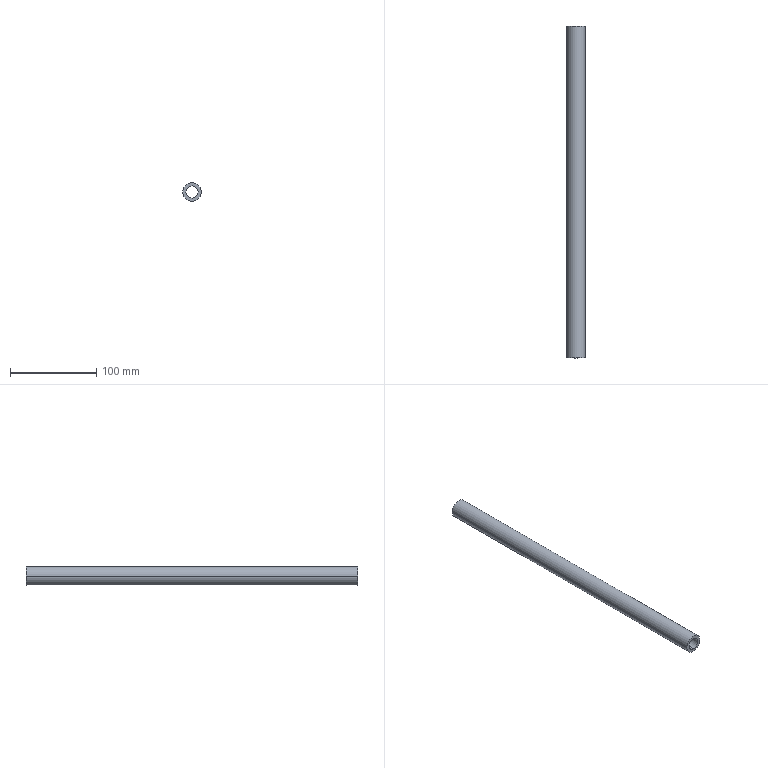Part | SolidWorks | features BaseBody 1 | 1 solid | 6 faces | box 21.234 x 384.346 x 21.234 mm | volume 76950 mm3 | plane 2 | spline 2 | cylinder 2 | commonest cylinder face diameters 21.234 x2
STEP:
#1=CARTESIAN_POINT('',(-35.306,422.7,7.));
#2=VERTEX_POINT('',#1);
#3=CARTESIAN_POINT('',(-35.306,422.7,-7.));
#4=VERTEX_POINT('',#3);
#5=CARTESIAN_POINT('',(-35.306,422.7,7.));
#6=CARTESIAN_POINT('',(-35.791,422.7,7.));
#7=CARTESIAN_POINT('',(-36.275,422.7,6.95));
#8=CARTESIAN_POINT('',(-36.75,422.7,6.85));
#9=CARTESIAN_POINT('',(-37.321,422.7,6.729));
#10=CARTESIAN_POINT('',(-37.875,422.7,6.538));
#11=CARTESIAN_POINT('',(-38.399,422.7,6.28));
#12=CARTESIAN_POINT('',(-39.149,422.7,5.91));
#13=CARTESIAN_POINT('',(-39.828,422.7,5.409));
#14=CARTESIAN_POINT('',(-40.401,422.7,4.8));
#15=CARTESIAN_POINT('',(-40.996,422.7,4.168));
#16=CARTESIAN_POINT('',(-41.469,422.7,3.431));
#17=CARTESIAN_POINT('',(-41.794,422.7,2.626));
#18=CARTESIAN_POINT('',(-42.132,422.7,1.792));
#19=CARTESIAN_POINT('',(-42.306,422.7,0.9002));
#20=CARTESIAN_POINT('',(-42.306,422.7,0.));
#21=CARTESIAN_POINT('',(-42.306,422.7,-0.9002));
#22=CARTESIAN_POINT('',(-42.132,422.7,-1.792));
#23=CARTESIAN_POINT('',(-41.794,422.7,-2.626));
#24=CARTESIAN_POINT('',(-41.469,422.7,-3.431));
#25=CARTESIAN_POINT('',(-40.996,422.7,-4.168));
#26=CARTESIAN_POINT('',(-40.401,422.7,-4.8));
#27=CARTESIAN_POINT('',(-39.828,422.7,-5.409));
#28=CARTESIAN_POINT('',(-39.149,422.7,-5.91));
#29=CARTESIAN_POINT('',(-38.399,422.7,-6.28));
#30=CARTESIAN_POINT('',(-37.875,422.7,-6.538));
#31=CARTESIAN_POINT('',(-37.321,422.7,-6.729));
#32=CARTESIAN_POINT('',(-36.75,422.7,-6.85));
#33=CARTESIAN_POINT('',(-36.275,422.7,-6.95));
#34=CARTESIAN_POINT('',(-35.791,422.7,-7.));
#35=CARTESIAN_POINT('',(-35.306,422.7,-7.));
#36=B_SPLINE_CURVE_WITH_KNOTS('',3,(#5,#6,#7,#8,#9,#10,#11,#12,#13,#14,#15,#16,#17,#18,#19,#20,#21,#22,#23,#24,#25,#26,#27,#28,#29,#30,#31,#32,#33,#34,#35),.UNSPECIFIED.,.F.,.F.,(4,3,3,3,3,3,3,3,3,3,4),(0.,0.1457,0.3209,0.572,0.8325,1.103,1.373,1.633,1.885,2.06,2.205),.UNSPECIFIED.);
#37=EDGE_CURVE('',#2,#4,#36,.T.);
#38=ORIENTED_EDGE('',*,*,#37,.F.);
#39=CARTESIAN_POINT('',(-35.306,422.7,-7.));
#40=CARTESIAN_POINT('',(-34.82,422.7,-7.));
#41=CARTESIAN_POINT('',(-34.336,422.7,-6.95));
#42=CARTESIAN_POINT('',(-33.861,422.7,-6.85));
#43=CARTESIAN_POINT('',(-33.29,422.7,-6.729));
#44=CARTESIAN_POINT('',(-32.736,422.7,-6.538));
#45=CARTESIAN_POINT('',(-32.212,422.7,-6.28));
#46=CARTESIAN_POINT('',(-31.462,422.7,-5.91));
#47=CARTESIAN_POINT('',(-30.784,422.7,-5.409));
#48=CARTESIAN_POINT('',(-30.21,422.7,-4.8));
#49=CARTESIAN_POINT('',(-29.615,422.7,-4.168));
#50=CARTESIAN_POINT('',(-29.142,422.7,-3.431));
#51=CARTESIAN_POINT('',(-28.817,422.7,-2.626));
#52=CARTESIAN_POINT('',(-28.479,422.7,-1.792));
#53=CARTESIAN_POINT('',(-28.305,422.7,-0.9002));
#54=CARTESIAN_POINT('',(-28.305,422.7,0.));
#55=CARTESIAN_POINT('',(-28.305,422.7,0.9002));
#56=CARTESIAN_POINT('',(-28.479,422.7,1.792));
#57=CARTESIAN_POINT('',(-28.817,422.7,2.626));
#58=CARTESIAN_POINT('',(-29.142,422.7,3.431));
#59=CARTESIAN_POINT('',(-29.615,422.7,4.168));
#60=CARTESIAN_POINT('',(-30.21,422.7,4.8));
#61=CARTESIAN_POINT('',(-30.784,422.7,5.409));
#62=CARTESIAN_POINT('',(-31.462,422.7,5.91));
#63=CARTESIAN_POINT('',(-32.212,422.7,6.28));
#64=CARTESIAN_POINT('',(-32.736,422.7,6.538));
#65=CARTESIAN_POINT('',(-33.29,422.7,6.729));
#66=CARTESIAN_POINT('',(-33.861,422.7,6.85));
#67=CARTESIAN_POINT('',(-34.336,422.7,6.95));
#68=CARTESIAN_POINT('',(-34.82,422.7,7.));
#69=CARTESIAN_POINT('',(-35.306,422.7,7.));
#70=B_SPLINE_CURVE_WITH_KNOTS('',3,(#39,#40,#41,#42,#43,#44,#45,#46,#47,#48,#49,#50,#51,#52,#53,#54,#55,#56,#57,#58,#59,#60,#61,#62,#63,#64,#65,#66,#67,#68,#69),.UNSPECIFIED.,.F.,.F.,(4,3,3,3,3,3,3,3,3,3,4),(0.,0.1457,0.3209,0.572,0.8325,1.103,1.373,1.633,1.885,2.06,2.205),.UNSPECIFIED.);
#71=EDGE_CURVE('',#4,#2,#70,.T.);
#72=ORIENTED_EDGE('',*,*,#71,.F.);
#73=EDGE_LOOP('',(#38,#72));
#74=FACE_BOUND('',#73,.T.);
#75=CARTESIAN_POINT('',(-24.689,422.7,0.));
#76=VERTEX_POINT('',#75);
#77=CARTESIAN_POINT('',(-45.923,422.7,0.));
#78=VERTEX_POINT('',#77);
#79=CARTESIAN_POINT('',(-35.306,422.7,0.));
#80=DIRECTION('',(0.,1.,0.));
#81=DIRECTION('',(1.,0.,0.));
#82=AXIS2_PLACEMENT_3D('',#79,#80,#81);
#83=CIRCLE('',#82,10.617);
#84=EDGE_CURVE('',#76,#78,#83,.T.);
#85=ORIENTED_EDGE('',*,*,#84,.F.);
#86=CARTESIAN_POINT('',(-35.306,422.7,0.));
#87=DIRECTION('',(0.,1.,0.));
#88=DIRECTION('',(-1.,0.,0.));
#89=AXIS2_PLACEMENT_3D('',#86,#87,#88);
#90=CIRCLE('',#89,10.617);
#91=EDGE_CURVE('',#78,#76,#90,.T.);
#92=ORIENTED_EDGE('',*,*,#91,.F.);
#93=EDGE_LOOP('',(#85,#92));
#94=FACE_OUTER_BOUND('',#93,.T.);
#95=CARTESIAN_POINT('',(-35.306,422.7,0.));
#96=DIRECTION('',(0.,-1.,0.));
#97=DIRECTION('',(0.,0.,-1.));
#98=AXIS2_PLACEMENT_3D('',#95,#96,#97);
#99=PLANE('',#98);
#100=ADVANCED_FACE('',(#74,#94),#99,.T.);
#101=CARTESIAN_POINT('',(-35.306,807.046,7.));
#102=VERTEX_POINT('',#101);
#103=CARTESIAN_POINT('',(-35.306,807.046,-7.));
#104=VERTEX_POINT('',#103);
#105=CARTESIAN_POINT('',(-35.306,807.046,7.));
#106=CARTESIAN_POINT('',(-34.82,807.046,7.));
#107=CARTESIAN_POINT('',(-34.336,807.046,6.95));
#108=CARTESIAN_POINT('',(-33.29,807.046,6.729));
#109=CARTESIAN_POINT('',(-32.736,807.046,6.538));
#110=CARTESIAN_POINT('',(-31.462,807.046,5.91));
#111=CARTESIAN_POINT('',(-30.784,807.046,5.409));
#112=CARTESIAN_POINT('',(-29.615,807.046,4.168));
#113=CARTESIAN_POINT('',(-29.142,807.046,3.431));
#114=CARTESIAN_POINT('',(-28.479,807.046,1.792));
#115=CARTESIAN_POINT('',(-28.305,807.046,0.9002));
#116=CARTESIAN_POINT('',(-28.305,807.046,-0.9002));
#117=CARTESIAN_POINT('',(-28.479,807.046,-1.792));
#118=CARTESIAN_POINT('',(-29.142,807.046,-3.431));
#119=CARTESIAN_POINT('',(-29.615,807.046,-4.168));
#120=CARTESIAN_POINT('',(-30.784,807.046,-5.409));
#121=CARTESIAN_POINT('',(-31.462,807.046,-5.91));
#122=CARTESIAN_POINT('',(-32.736,807.046,-6.538));
#123=CARTESIAN_POINT('',(-33.29,807.046,-6.729));
#124=CARTESIAN_POINT('',(-34.336,807.046,-6.95));
#125=CARTESIAN_POINT('',(-34.82,807.046,-7.));
#126=CARTESIAN_POINT('',(-35.306,807.046,-7.));
#127=B_SPLINE_CURVE_WITH_KNOTS('',3,(#105,#106,#107,#108,#109,#110,#111,#112,#113,#114,#115,#116,#117,#118,#119,#120,#121,#122,#123,#124,#125,#126),.UNSPECIFIED.,.F.,.F.,(4,2,2,2,2,2,2,2,2,2,4),(0.,0.1456,0.3207,0.5718,0.8321,1.102,1.372,1.633,1.884,2.059,2.204),.UNSPECIFIED.);
#128=EDGE_CURVE('',#102,#104,#127,.T.);
#129=ORIENTED_EDGE('',*,*,#128,.F.);
#130=CARTESIAN_POINT('',(-35.306,807.046,-7.));
#131=CARTESIAN_POINT('',(-35.791,807.046,-7.));
#132=CARTESIAN_POINT('',(-36.275,807.046,-6.95));
#133=CARTESIAN_POINT('',(-36.75,807.046,-6.85));
#134=CARTESIAN_POINT('',(-37.321,807.046,-6.729));
#135=CARTESIAN_POINT('',(-37.875,807.046,-6.538));
#136=CARTESIAN_POINT('',(-38.399,807.046,-6.28));
#137=CARTESIAN_POINT('',(-39.149,807.046,-5.91));
#138=CARTESIAN_POINT('',(-39.828,807.046,-5.409));
#139=CARTESIAN_POINT('',(-40.401,807.046,-4.8));
#140=CARTESIAN_POINT('',(-40.996,807.046,-4.168));
#141=CARTESIAN_POINT('',(-41.469,807.046,-3.431));
#142=CARTESIAN_POINT('',(-41.794,807.046,-2.626));
#143=CARTESIAN_POINT('',(-42.132,807.046,-1.792));
#144=CARTESIAN_POINT('',(-42.306,807.046,-0.9002));
#145=CARTESIAN_POINT('',(-42.306,807.046,0.));
#146=CARTESIAN_POINT('',(-42.306,807.046,0.9002));
#147=CARTESIAN_POINT('',(-42.132,807.046,1.792));
#148=CARTESIAN_POINT('',(-41.794,807.046,2.626));
#149=CARTESIAN_POINT('',(-41.469,807.046,3.431));
#150=CARTESIAN_POINT('',(-40.996,807.046,4.168));
#151=CARTESIAN_POINT('',(-40.401,807.046,4.8));
#152=CARTESIAN_POINT('',(-39.828,807.046,5.409));
#153=CARTESIAN_POINT('',(-39.149,807.046,5.91));
#154=CARTESIAN_POINT('',(-38.399,807.046,6.28));
#155=CARTESIAN_POINT('',(-37.875,807.046,6.538));
#156=CARTESIAN_POINT('',(-37.321,807.046,6.729));
#157=CARTESIAN_POINT('',(-36.75,807.046,6.85));
#158=CARTESIAN_POINT('',(-36.275,807.046,6.95));
#159=CARTESIAN_POINT('',(-35.791,807.046,7.));
#160=CARTESIAN_POINT('',(-35.306,807.046,7.));
#161=B_SPLINE_CURVE_WITH_KNOTS('',3,(#130,#131,#132,#133,#134,#135,#136,#137,#138,#139,#140,#141,#142,#143,#144,#145,#146,#147,#148,#149,#150,#151,#152,#153,#154,#155,#156,#157,#158,#159,#160),.UNSPECIFIED.,.F.,.F.,(4,3,3,3,3,3,3,3,3,3,4),(0.,0.1456,0.3207,0.5718,0.8321,1.102,1.372,1.633,1.884,2.059,2.204),.UNSPECIFIED.);
#162=EDGE_CURVE('',#104,#102,#161,.T.);
#163=ORIENTED_EDGE('',*,*,#162,.F.);
#164=EDGE_LOOP('',(#129,#163));
#165=FACE_BOUND('',#164,.T.);
#166=CARTESIAN_POINT('',(-24.689,807.046,0.));
#167=VERTEX_POINT('',#166);
#168=CARTESIAN_POINT('',(-45.923,807.046,0.));
#169=VERTEX_POINT('',#168);
#170=CARTESIAN_POINT('',(-35.306,807.046,0.));
#171=DIRECTION('',(0.,-1.,0.));
#172=DIRECTION('',(1.,0.,0.));
#173=AXIS2_PLACEMENT_3D('',#170,#171,#172);
#174=CIRCLE('',#173,10.617);
#175=EDGE_CURVE('',#167,#169,#174,.T.);
#176=ORIENTED_EDGE('',*,*,#175,.F.);
#177=CARTESIAN_POINT('',(-35.306,807.046,0.));
#178=DIRECTION('',(0.,-1.,0.));
#179=DIRECTION('',(-1.,0.,0.));
#180=AXIS2_PLACEMENT_3D('',#177,#178,#179);
#181=CIRCLE('',#180,10.617);
#182=EDGE_CURVE('',#169,#167,#181,.T.);
#183=ORIENTED_EDGE('',*,*,#182,.F.);
#184=EDGE_LOOP('',(#176,#183));
#185=FACE_OUTER_BOUND('',#184,.T.);
#186=CARTESIAN_POINT('',(-35.306,807.046,0.));
#187=DIRECTION('',(0.,1.,0.));
#188=DIRECTION('',(1.,0.,0.));
#189=AXIS2_PLACEMENT_3D('',#186,#187,#188);
#190=PLANE('',#189);
#191=ADVANCED_FACE('',(#165,#185),#190,.T.);
#192=ORIENTED_EDGE('',*,*,#71,.T.);
#193=CARTESIAN_POINT('',(-35.306,807.046,7.));
#194=DIRECTION('',(0.,-1.,0.));
#195=VECTOR('',#194,1000.);
#196=LINE('',#193,#195);
#197=EDGE_CURVE('',#102,#2,#196,.T.);
#198=ORIENTED_EDGE('',*,*,#197,.F.);
#199=ORIENTED_EDGE('',*,*,#128,.T.);
#200=CARTESIAN_POINT('',(-35.306,422.7,-7.));
#201=DIRECTION('',(0.,1.,0.));
#202=VECTOR('',#201,1000.);
#203=LINE('',#200,#202);
#204=EDGE_CURVE('',#4,#104,#203,.T.);
#205=ORIENTED_EDGE('',*,*,#204,.F.);
#206=EDGE_LOOP('',(#192,#198,#199,#205));
#207=FACE_OUTER_BOUND('',#206,.T.);
#208=CARTESIAN_POINT('',(-35.306,807.046,7.));
#209=CARTESIAN_POINT('',(-35.306,384.265,7.));
#210=CARTESIAN_POINT('',(-34.82,807.046,7.));
#211=CARTESIAN_POINT('',(-34.82,384.265,7.));
#212=CARTESIAN_POINT('',(-34.336,807.046,6.95));
#213=CARTESIAN_POINT('',(-34.336,384.265,6.95));
#214=CARTESIAN_POINT('',(-33.29,807.046,6.729));
#215=CARTESIAN_POINT('',(-33.29,384.265,6.729));
#216=CARTESIAN_POINT('',(-32.736,807.046,6.538));
#217=CARTESIAN_POINT('',(-32.736,384.265,6.538));
#218=CARTESIAN_POINT('',(-31.462,807.046,5.91));
#219=CARTESIAN_POINT('',(-31.462,384.265,5.91));
#220=CARTESIAN_POINT('',(-30.784,807.046,5.409));
#221=CARTESIAN_POINT('',(-30.784,384.265,5.409));
#222=CARTESIAN_POINT('',(-29.615,807.046,4.168));
#223=CARTESIAN_POINT('',(-29.615,384.265,4.168));
#224=CARTESIAN_POINT('',(-29.142,807.046,3.431));
#225=CARTESIAN_POINT('',(-29.142,384.265,3.431));
#226=CARTESIAN_POINT('',(-28.479,807.046,1.792));
#227=CARTESIAN_POINT('',(-28.479,384.265,1.792));
#228=CARTESIAN_POINT('',(-28.305,807.046,0.9002));
#229=CARTESIAN_POINT('',(-28.305,384.265,0.9002));
#230=CARTESIAN_POINT('',(-28.305,807.046,-0.9002));
#231=CARTESIAN_POINT('',(-28.305,384.265,-0.9002));
#232=CARTESIAN_POINT('',(-28.479,807.046,-1.792));
#233=CARTESIAN_POINT('',(-28.479,384.265,-1.792));
#234=CARTESIAN_POINT('',(-29.142,807.046,-3.431));
#235=CARTESIAN_POINT('',(-29.142,384.265,-3.431));
#236=CARTESIAN_POINT('',(-29.615,807.046,-4.168));
#237=CARTESIAN_POINT('',(-29.615,384.265,-4.168));
#238=CARTESIAN_POINT('',(-30.784,807.046,-5.409));
#239=CARTESIAN_POINT('',(-30.784,384.265,-5.409));
#240=CARTESIAN_POINT('',(-31.462,807.046,-5.91));
#241=CARTESIAN_POINT('',(-31.462,384.265,-5.91));
#242=CARTESIAN_POINT('',(-32.736,807.046,-6.538));
#243=CARTESIAN_POINT('',(-32.736,384.265,-6.538));
#244=CARTESIAN_POINT('',(-33.29,807.046,-6.729));
#245=CARTESIAN_POINT('',(-33.29,384.265,-6.729));
#246=CARTESIAN_POINT('',(-34.336,807.046,-6.95));
#247=CARTESIAN_POINT('',(-34.336,384.265,-6.95));
#248=CARTESIAN_POINT('',(-34.82,807.046,-7.));
#249=CARTESIAN_POINT('',(-34.82,384.265,-7.));
#250=CARTESIAN_POINT('',(-35.306,807.046,-7.));
#251=CARTESIAN_POINT('',(-35.306,384.265,-7.));
#252=B_SPLINE_SURFACE_WITH_KNOTS('',3,1,((#208,#209),(#210,#211),(#212,#213),(#214,#215),(#216,#217),(#218,#219),(#220,#221),(#222,#223),(#224,#225),(#226,#227),(#228,#229),(#230,#231),(#232,#233),(#234,#235),(#236,#237),(#238,#239),(#240,#241),(#242,#243),(#244,#245),(#246,#247),(#248,#249),(#250,#251)),.UNSPECIFIED.,.F.,.F.,.F.,(4,2,2,2,2,2,2,2,2,2,4),(2,2),(0.000001,0.1456,0.3207,0.5718,0.8321,1.102,1.372,1.633,1.884,2.059,2.204),(0.,42.278),.UNSPECIFIED.);
#253=ADVANCED_FACE('',(#207),#252,.T.);
#254=ORIENTED_EDGE('',*,*,#91,.T.);
#255=CARTESIAN_POINT('',(-24.689,807.046,0.));
#256=DIRECTION('',(0.,-1.,0.));
#257=VECTOR('',#256,1000.);
#258=LINE('',#255,#257);
#259=EDGE_CURVE('',#167,#76,#258,.T.);
#260=ORIENTED_EDGE('',*,*,#259,.F.);
#261=ORIENTED_EDGE('',*,*,#175,.T.);
#262=CARTESIAN_POINT('',(-45.923,422.7,0.));
#263=DIRECTION('',(0.,1.,0.));
#264=VECTOR('',#263,1000.);
#265=LINE('',#262,#264);
#266=EDGE_CURVE('',#78,#169,#265,.T.);
#267=ORIENTED_EDGE('',*,*,#266,.F.);
#268=EDGE_LOOP('',(#254,#260,#261,#267));
#269=FACE_OUTER_BOUND('',#268,.T.);
#270=CARTESIAN_POINT('',(-35.306,807.046,0.));
#271=DIRECTION('',(0.,-1.,0.));
#272=DIRECTION('',(1.,0.,0.));
#273=AXIS2_PLACEMENT_3D('',#270,#271,#272);
#274=CYLINDRICAL_SURFACE('',#273,10.617);
#275=ADVANCED_FACE('',(#269),#274,.T.);
#276=ORIENTED_EDGE('',*,*,#266,.T.);
#277=ORIENTED_EDGE('',*,*,#182,.T.);
#278=ORIENTED_EDGE('',*,*,#259,.T.);
#279=ORIENTED_EDGE('',*,*,#84,.T.);
#280=EDGE_LOOP('',(#276,#277,#278,#279));
#281=FACE_OUTER_BOUND('',#280,.T.);
#282=CARTESIAN_POINT('',(-35.306,807.046,0.));
#283=DIRECTION('',(0.,-1.,0.));
#284=DIRECTION('',(1.,0.,0.));
#285=AXIS2_PLACEMENT_3D('',#282,#283,#284);
#286=CYLINDRICAL_SURFACE('',#285,10.617);
#287=ADVANCED_FACE('',(#281),#286,.T.);
#288=ORIENTED_EDGE('',*,*,#37,.T.);
#289=ORIENTED_EDGE('',*,*,#204,.T.);
#290=ORIENTED_EDGE('',*,*,#162,.T.);
#291=ORIENTED_EDGE('',*,*,#197,.T.);
#292=EDGE_LOOP('',(#288,#289,#290,#291));
#293=FACE_OUTER_BOUND('',#292,.T.);
#294=CARTESIAN_POINT('',(-35.306,807.046,-7.));
#295=CARTESIAN_POINT('',(-35.306,384.265,-7.));
#296=CARTESIAN_POINT('',(-35.791,807.046,-7.));
#297=CARTESIAN_POINT('',(-35.791,384.265,-7.));
#298=CARTESIAN_POINT('',(-36.275,807.046,-6.95));
#299=CARTESIAN_POINT('',(-36.275,384.265,-6.95));
#300=CARTESIAN_POINT('',(-37.321,807.046,-6.729));
#301=CARTESIAN_POINT('',(-37.321,384.265,-6.729));
#302=CARTESIAN_POINT('',(-37.875,807.046,-6.538));
#303=CARTESIAN_POINT('',(-37.875,384.265,-6.538));
#304=CARTESIAN_POINT('',(-39.149,807.046,-5.91));
#305=CARTESIAN_POINT('',(-39.149,384.265,-5.91));
#306=CARTESIAN_POINT('',(-39.828,807.046,-5.409));
#307=CARTESIAN_POINT('',(-39.828,384.265,-5.409));
#308=CARTESIAN_POINT('',(-40.996,807.046,-4.168));
#309=CARTESIAN_POINT('',(-40.996,384.265,-4.168));
#310=CARTESIAN_POINT('',(-41.469,807.046,-3.431));
#311=CARTESIAN_POINT('',(-41.469,384.265,-3.431));
#312=CARTESIAN_POINT('',(-42.132,807.046,-1.792));
#313=CARTESIAN_POINT('',(-42.132,384.265,-1.792));
#314=CARTESIAN_POINT('',(-42.306,807.046,-0.9002));
#315=CARTESIAN_POINT('',(-42.306,384.265,-0.9002));
#316=CARTESIAN_POINT('',(-42.306,807.046,0.9002));
#317=CARTESIAN_POINT('',(-42.306,384.265,0.9002));
#318=CARTESIAN_POINT('',(-42.132,807.046,1.792));
#319=CARTESIAN_POINT('',(-42.132,384.265,1.792));
#320=CARTESIAN_POINT('',(-41.469,807.046,3.431));
#321=CARTESIAN_POINT('',(-41.469,384.265,3.431));
#322=CARTESIAN_POINT('',(-40.996,807.046,4.168));
#323=CARTESIAN_POINT('',(-40.996,384.265,4.168));
#324=CARTESIAN_POINT('',(-39.828,807.046,5.409));
#325=CARTESIAN_POINT('',(-39.828,384.265,5.409));
#326=CARTESIAN_POINT('',(-39.149,807.046,5.91));
#327=CARTESIAN_POINT('',(-39.149,384.265,5.91));
#328=CARTESIAN_POINT('',(-37.875,807.046,6.538));
#329=CARTESIAN_POINT('',(-37.875,384.265,6.538));
#330=CARTESIAN_POINT('',(-37.321,807.046,6.729));
#331=CARTESIAN_POINT('',(-37.321,384.265,6.729));
#332=CARTESIAN_POINT('',(-36.275,807.046,6.95));
#333=CARTESIAN_POINT('',(-36.275,384.265,6.95));
#334=CARTESIAN_POINT('',(-35.791,807.046,7.));
#335=CARTESIAN_POINT('',(-35.791,384.265,7.));
#336=CARTESIAN_POINT('',(-35.306,807.046,7.));
#337=CARTESIAN_POINT('',(-35.306,384.265,7.));
#338=B_SPLINE_SURFACE_WITH_KNOTS('',3,1,((#294,#295),(#296,#297),(#298,#299),(#300,#301),(#302,#303),(#304,#305),(#306,#307),(#308,#309),(#310,#311),(#312,#313),(#314,#315),(#316,#317),(#318,#319),(#320,#321),(#322,#323),(#324,#325),(#326,#327),(#328,#329),(#330,#331),(#332,#333),(#334,#335),(#336,#337)),.UNSPECIFIED.,.F.,.F.,.F.,(4,2,2,2,2,2,2,2,2,2,4),(2,2),(0.000001,0.1456,0.3207,0.5718,0.8321,1.102,1.372,1.633,1.884,2.059,2.204),(0.,42.278),.UNSPECIFIED.);
#339=ADVANCED_FACE('',(#293),#338,.T.);
#340=CLOSED_SHELL('',(#100,#191,#253,#275,#287,#339));
#341=MANIFOLD_SOLID_BREP('',#340);
#342=CARTESIAN_POINT('',(0.,0.,0.));
#343=DIRECTION('',(0.,0.,1.));
#344=DIRECTION('',(1.,0.,0.));
#345=AXIS2_PLACEMENT_3D('',#342,#343,#344);
#346=(LENGTH_UNIT()NAMED_UNIT(*)SI_UNIT(.MILLI.,.METRE.));
#347=UNCERTAINTY_MEASURE_WITH_UNIT(LENGTH_MEASURE(0.00001),#346,'','');
#348=(NAMED_UNIT(*)PLANE_ANGLE_UNIT()SI_UNIT($,.RADIAN.));
#349=(NAMED_UNIT(*)SI_UNIT($,.STERADIAN.)SOLID_ANGLE_UNIT());
#350=(GEOMETRIC_REPRESENTATION_CONTEXT(3)GLOBAL_UNCERTAINTY_ASSIGNED_CONTEXT((#347))GLOBAL_UNIT_ASSIGNED_CONTEXT((#346,#348,#349))REPRESENTATION_CONTEXT('',''));
#351=ADVANCED_BREP_SHAPE_REPRESENTATION('',(#341,#345),#350);